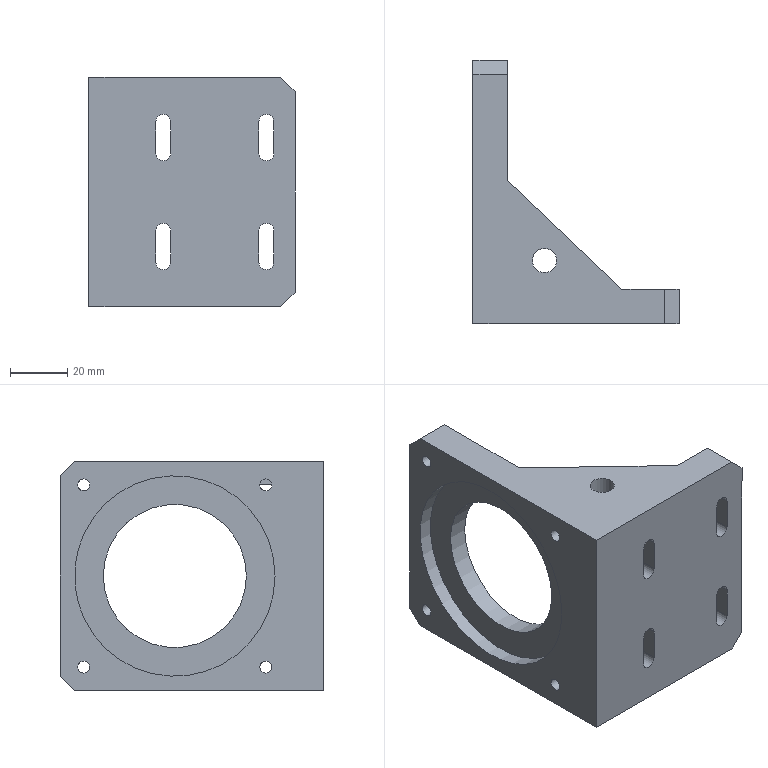Part | NX | 1 solid | 39 faces | box 72 x 92 x 80 mm | volume 113529 mm3 | plane 24 | cylinder 15 | commonest cylinder face diameters 5.2 x8 4.2 x4 8.5 x1 50 x1 70 x1
STEP:
#1=CARTESIAN_POINT('',(0.,65.,0.));
#2=VERTEX_POINT('',#1);
#3=CARTESIAN_POINT('',(0.,40.,0.));
#4=DIRECTION('',(1.,0.,0.));
#5=DIRECTION('',(0.,1.,0.));
#6=AXIS2_PLACEMENT_3D('',#3,#4,#5);
#7=CIRCLE('',#6,25.);
#8=EDGE_CURVE('',#2,#2,#7,.T.);
#9=ORIENTED_EDGE('',*,*,#8,.T.);
#10=EDGE_LOOP('',(#9));
#11=FACE_BOUND('',#10,.T.);
#12=CARTESIAN_POINT('',(-7.,15.,0.));
#13=VERTEX_POINT('',#12);
#14=CARTESIAN_POINT('',(-7.,40.,0.));
#15=DIRECTION('',(-1.,0.,0.));
#16=DIRECTION('',(0.,-1.,0.));
#17=AXIS2_PLACEMENT_3D('',#14,#15,#16);
#18=CIRCLE('',#17,25.);
#19=EDGE_CURVE('',#13,#13,#18,.F.);
#20=ORIENTED_EDGE('',*,*,#19,.F.);
#21=EDGE_LOOP('',(#20));
#22=FACE_BOUND('',#21,.T.);
#23=CARTESIAN_POINT('',(60.,40.,0.));
#24=DIRECTION('',(-1.,0.,0.));
#25=DIRECTION('',(0.,-1.,0.));
#26=AXIS2_PLACEMENT_3D('',#23,#24,#25);
#27=CYLINDRICAL_SURFACE('',#26,25.);
#28=ADVANCED_FACE('',(#11,#22),#27,.F.);
#29=CARTESIAN_POINT('',(0.,38.,32.));
#30=VERTEX_POINT('',#29);
#31=CARTESIAN_POINT('',(0.,10.272,32.));
#32=VERTEX_POINT('',#31);
#33=CARTESIAN_POINT('',(0.,80.,32.));
#34=DIRECTION('',(0.,-1.,0.));
#35=VECTOR('',#34,1000.);
#36=LINE('',#33,#35);
#37=EDGE_CURVE('',#30,#32,#36,.T.);
#38=ORIENTED_EDGE('',*,*,#37,.T.);
#39=CARTESIAN_POINT('',(0.,6.088,32.));
#40=VERTEX_POINT('',#39);
#41=CARTESIAN_POINT('',(0.,8.18,31.82));
#42=DIRECTION('',(1.,0.,0.));
#43=DIRECTION('',(0.,1.,0.));
#44=AXIS2_PLACEMENT_3D('',#41,#42,#43);
#45=CIRCLE('',#44,2.1);
#46=EDGE_CURVE('',#32,#40,#45,.F.);
#47=ORIENTED_EDGE('',*,*,#46,.T.);
#48=CARTESIAN_POINT('',(0.,0.,32.));
#49=VERTEX_POINT('',#48);
#50=CARTESIAN_POINT('',(0.,80.,32.));
#51=DIRECTION('',(0.,-1.,0.));
#52=VECTOR('',#51,1000.);
#53=LINE('',#50,#52);
#54=EDGE_CURVE('',#40,#49,#53,.T.);
#55=ORIENTED_EDGE('',*,*,#54,.T.);
#56=CARTESIAN_POINT('',(0.,0.,-40.));
#57=VERTEX_POINT('',#56);
#58=CARTESIAN_POINT('',(0.,0.,40.));
#59=DIRECTION('',(0.,0.,-1.));
#60=VECTOR('',#59,1000.);
#61=LINE('',#58,#60);
#62=EDGE_CURVE('',#49,#57,#61,.T.);
#63=ORIENTED_EDGE('',*,*,#62,.T.);
#64=CARTESIAN_POINT('',(0.,75.,-40.));
#65=VERTEX_POINT('',#64);
#66=CARTESIAN_POINT('',(0.,80.,-40.));
#67=DIRECTION('',(0.,-1.,0.));
#68=VECTOR('',#67,1000.);
#69=LINE('',#66,#68);
#70=EDGE_CURVE('',#65,#57,#69,.T.);
#71=ORIENTED_EDGE('',*,*,#70,.F.);
#72=CARTESIAN_POINT('',(0.,80.,-35.));
#73=VERTEX_POINT('',#72);
#74=CARTESIAN_POINT('',(0.,117.5,2.5));
#75=DIRECTION('',(0.,-0.7071,-0.7071));
#76=VECTOR('',#75,1000.);
#77=LINE('',#74,#76);
#78=EDGE_CURVE('',#65,#73,#77,.F.);
#79=ORIENTED_EDGE('',*,*,#78,.T.);
#80=CARTESIAN_POINT('',(0.,80.,35.));
#81=VERTEX_POINT('',#80);
#82=CARTESIAN_POINT('',(0.,80.,40.));
#83=DIRECTION('',(0.,0.,-1.));
#84=VECTOR('',#83,1000.);
#85=LINE('',#82,#84);
#86=EDGE_CURVE('',#81,#73,#85,.T.);
#87=ORIENTED_EDGE('',*,*,#86,.F.);
#88=CARTESIAN_POINT('',(0.,75.,40.));
#89=VERTEX_POINT('',#88);
#90=CARTESIAN_POINT('',(0.,77.5,37.5));
#91=DIRECTION('',(0.,-0.7071,0.7071));
#92=VECTOR('',#91,1000.);
#93=LINE('',#90,#92);
#94=EDGE_CURVE('',#81,#89,#93,.T.);
#95=ORIENTED_EDGE('',*,*,#94,.T.);
#96=CARTESIAN_POINT('',(0.,38.,40.));
#97=VERTEX_POINT('',#96);
#98=CARTESIAN_POINT('',(0.,80.,40.));
#99=DIRECTION('',(0.,-1.,0.));
#100=VECTOR('',#99,1000.);
#101=LINE('',#98,#100);
#102=EDGE_CURVE('',#89,#97,#101,.T.);
#103=ORIENTED_EDGE('',*,*,#102,.T.);
#104=CARTESIAN_POINT('',(0.,38.,40.));
#105=DIRECTION('',(0.,0.,-1.));
#106=VECTOR('',#105,1000.);
#107=LINE('',#104,#106);
#108=EDGE_CURVE('',#30,#97,#107,.F.);
#109=ORIENTED_EDGE('',*,*,#108,.F.);
#110=EDGE_LOOP('',(#38,#47,#55,#63,#71,#79,#87,#95,#103,#109));
#111=FACE_BOUND('',#110,.T.);
#112=CARTESIAN_POINT('',(0.,10.28,-31.82));
#113=VERTEX_POINT('',#112);
#114=CARTESIAN_POINT('',(0.,8.18,-31.82));
#115=DIRECTION('',(1.,0.,0.));
#116=DIRECTION('',(0.,1.,0.));
#117=AXIS2_PLACEMENT_3D('',#114,#115,#116);
#118=CIRCLE('',#117,2.1);
#119=EDGE_CURVE('',#113,#113,#118,.F.);
#120=ORIENTED_EDGE('',*,*,#119,.T.);
#121=EDGE_LOOP('',(#120));
#122=FACE_BOUND('',#121,.T.);
#123=ORIENTED_EDGE('',*,*,#8,.F.);
#124=EDGE_LOOP('',(#123));
#125=FACE_BOUND('',#124,.T.);
#126=CARTESIAN_POINT('',(0.,73.92,31.82));
#127=VERTEX_POINT('',#126);
#128=CARTESIAN_POINT('',(0.,71.82,31.82));
#129=DIRECTION('',(1.,0.,0.));
#130=DIRECTION('',(0.,1.,0.));
#131=AXIS2_PLACEMENT_3D('',#128,#129,#130);
#132=CIRCLE('',#131,2.1);
#133=EDGE_CURVE('',#127,#127,#132,.F.);
#134=ORIENTED_EDGE('',*,*,#133,.T.);
#135=EDGE_LOOP('',(#134));
#136=FACE_BOUND('',#135,.T.);
#137=CARTESIAN_POINT('',(0.,73.92,-31.82));
#138=VERTEX_POINT('',#137);
#139=CARTESIAN_POINT('',(0.,71.82,-31.82));
#140=DIRECTION('',(1.,0.,0.));
#141=DIRECTION('',(0.,1.,0.));
#142=AXIS2_PLACEMENT_3D('',#139,#140,#141);
#143=CIRCLE('',#142,2.1);
#144=EDGE_CURVE('',#138,#138,#143,.F.);
#145=ORIENTED_EDGE('',*,*,#144,.T.);
#146=EDGE_LOOP('',(#145));
#147=FACE_BOUND('',#146,.T.);
#148=CARTESIAN_POINT('',(0.,80.,40.));
#149=DIRECTION('',(1.,0.,0.));
#150=DIRECTION('',(0.,1.,0.));
#151=AXIS2_PLACEMENT_3D('',#148,#149,#150);
#152=PLANE('',#151);
#153=ADVANCED_FACE('',(#111,#122,#125,#136,#147),#152,.T.);
#154=CARTESIAN_POINT('',(52.6,-12.,24.5));
#155=VERTEX_POINT('',#154);
#156=CARTESIAN_POINT('',(52.6,-12.,13.5));
#157=VERTEX_POINT('',#156);
#158=CARTESIAN_POINT('',(52.6,-12.,13.5));
#159=DIRECTION('',(0.,0.,-1.));
#160=VECTOR('',#159,1000.);
#161=LINE('',#158,#160);
#162=EDGE_CURVE('',#155,#157,#161,.T.);
#163=ORIENTED_EDGE('',*,*,#162,.T.);
#164=CARTESIAN_POINT('',(47.4,-12.,13.5));
#165=VERTEX_POINT('',#164);
#166=CARTESIAN_POINT('',(50.,-12.,13.5));
#167=DIRECTION('',(0.,1.,0.));
#168=DIRECTION('',(0.,0.,1.));
#169=AXIS2_PLACEMENT_3D('',#166,#167,#168);
#170=CIRCLE('',#169,2.6);
#171=EDGE_CURVE('',#157,#165,#170,.T.);
#172=ORIENTED_EDGE('',*,*,#171,.T.);
#173=CARTESIAN_POINT('',(47.4,-12.,24.5));
#174=VERTEX_POINT('',#173);
#175=CARTESIAN_POINT('',(47.4,-12.,13.5));
#176=DIRECTION('',(0.,0.,1.));
#177=VECTOR('',#176,1000.);
#178=LINE('',#175,#177);
#179=EDGE_CURVE('',#165,#174,#178,.T.);
#180=ORIENTED_EDGE('',*,*,#179,.T.);
#181=CARTESIAN_POINT('',(50.,-12.,24.5));
#182=DIRECTION('',(0.,1.,0.));
#183=DIRECTION('',(0.,0.,1.));
#184=AXIS2_PLACEMENT_3D('',#181,#182,#183);
#185=CIRCLE('',#184,2.6);
#186=EDGE_CURVE('',#174,#155,#185,.T.);
#187=ORIENTED_EDGE('',*,*,#186,.T.);
#188=EDGE_LOOP('',(#163,#172,#180,#187));
#189=FACE_BOUND('',#188,.T.);
#190=CARTESIAN_POINT('',(16.6,-12.,24.5));
#191=VERTEX_POINT('',#190);
#192=CARTESIAN_POINT('',(16.6,-12.,13.5));
#193=VERTEX_POINT('',#192);
#194=CARTESIAN_POINT('',(16.6,-12.,13.5));
#195=DIRECTION('',(0.,0.,-1.));
#196=VECTOR('',#195,1000.);
#197=LINE('',#194,#196);
#198=EDGE_CURVE('',#191,#193,#197,.T.);
#199=ORIENTED_EDGE('',*,*,#198,.T.);
#200=CARTESIAN_POINT('',(11.4,-12.,13.5));
#201=VERTEX_POINT('',#200);
#202=CARTESIAN_POINT('',(14.,-12.,13.5));
#203=DIRECTION('',(0.,1.,0.));
#204=DIRECTION('',(0.,0.,1.));
#205=AXIS2_PLACEMENT_3D('',#202,#203,#204);
#206=CIRCLE('',#205,2.6);
#207=EDGE_CURVE('',#193,#201,#206,.T.);
#208=ORIENTED_EDGE('',*,*,#207,.T.);
#209=CARTESIAN_POINT('',(11.4,-12.,24.5));
#210=VERTEX_POINT('',#209);
#211=CARTESIAN_POINT('',(11.4,-12.,13.5));
#212=DIRECTION('',(0.,0.,1.));
#213=VECTOR('',#212,1000.);
#214=LINE('',#211,#213);
#215=EDGE_CURVE('',#201,#210,#214,.T.);
#216=ORIENTED_EDGE('',*,*,#215,.T.);
#217=CARTESIAN_POINT('',(14.,-12.,24.5));
#218=DIRECTION('',(0.,1.,0.));
#219=DIRECTION('',(0.,0.,1.));
#220=AXIS2_PLACEMENT_3D('',#217,#218,#219);
#221=CIRCLE('',#220,2.6);
#222=EDGE_CURVE('',#210,#191,#221,.T.);
#223=ORIENTED_EDGE('',*,*,#222,.T.);
#224=EDGE_LOOP('',(#199,#208,#216,#223));
#225=FACE_BOUND('',#224,.T.);
#226=CARTESIAN_POINT('',(47.4,-12.,-24.5));
#227=VERTEX_POINT('',#226);
#228=CARTESIAN_POINT('',(47.4,-12.,-13.5));
#229=VERTEX_POINT('',#228);
#230=CARTESIAN_POINT('',(47.4,-12.,-13.5));
#231=DIRECTION('',(0.,0.,1.));
#232=VECTOR('',#231,1000.);
#233=LINE('',#230,#232);
#234=EDGE_CURVE('',#227,#229,#233,.T.);
#235=ORIENTED_EDGE('',*,*,#234,.T.);
#236=CARTESIAN_POINT('',(52.6,-12.,-13.5));
#237=VERTEX_POINT('',#236);
#238=CARTESIAN_POINT('',(50.,-12.,-13.5));
#239=DIRECTION('',(0.,1.,0.));
#240=DIRECTION('',(0.,0.,1.));
#241=AXIS2_PLACEMENT_3D('',#238,#239,#240);
#242=CIRCLE('',#241,2.6);
#243=EDGE_CURVE('',#229,#237,#242,.T.);
#244=ORIENTED_EDGE('',*,*,#243,.T.);
#245=CARTESIAN_POINT('',(52.6,-12.,-24.5));
#246=VERTEX_POINT('',#245);
#247=CARTESIAN_POINT('',(52.6,-12.,-13.5));
#248=DIRECTION('',(0.,0.,-1.));
#249=VECTOR('',#248,1000.);
#250=LINE('',#247,#249);
#251=EDGE_CURVE('',#237,#246,#250,.T.);
#252=ORIENTED_EDGE('',*,*,#251,.T.);
#253=CARTESIAN_POINT('',(50.,-12.,-24.5));
#254=DIRECTION('',(0.,1.,0.));
#255=DIRECTION('',(0.,0.,1.));
#256=AXIS2_PLACEMENT_3D('',#253,#254,#255);
#257=CIRCLE('',#256,2.6);
#258=EDGE_CURVE('',#246,#227,#257,.T.);
#259=ORIENTED_EDGE('',*,*,#258,.T.);
#260=EDGE_LOOP('',(#235,#244,#252,#259));
#261=FACE_BOUND('',#260,.T.);
#262=CARTESIAN_POINT('',(16.6,-12.,-13.5));
#263=VERTEX_POINT('',#262);
#264=CARTESIAN_POINT('',(16.6,-12.,-24.5));
#265=VERTEX_POINT('',#264);
#266=CARTESIAN_POINT('',(16.6,-12.,-24.5));
#267=DIRECTION('',(0.,0.,-1.));
#268=VECTOR('',#267,1000.);
#269=LINE('',#266,#268);
#270=EDGE_CURVE('',#263,#265,#269,.T.);
#271=ORIENTED_EDGE('',*,*,#270,.T.);
#272=CARTESIAN_POINT('',(11.4,-12.,-24.5));
#273=VERTEX_POINT('',#272);
#274=CARTESIAN_POINT('',(14.,-12.,-24.5));
#275=DIRECTION('',(0.,1.,0.));
#276=DIRECTION('',(0.,0.,1.));
#277=AXIS2_PLACEMENT_3D('',#274,#275,#276);
#278=CIRCLE('',#277,2.6);
#279=EDGE_CURVE('',#265,#273,#278,.T.);
#280=ORIENTED_EDGE('',*,*,#279,.T.);
#281=CARTESIAN_POINT('',(11.4,-12.,-13.5));
#282=VERTEX_POINT('',#281);
#283=CARTESIAN_POINT('',(11.4,-12.,-24.5));
#284=DIRECTION('',(0.,0.,1.));
#285=VECTOR('',#284,1000.);
#286=LINE('',#283,#285);
#287=EDGE_CURVE('',#273,#282,#286,.T.);
#288=ORIENTED_EDGE('',*,*,#287,.T.);
#289=CARTESIAN_POINT('',(14.,-12.,-13.5));
#290=DIRECTION('',(0.,1.,0.));
#291=DIRECTION('',(0.,0.,1.));
#292=AXIS2_PLACEMENT_3D('',#289,#290,#291);
#293=CIRCLE('',#292,2.6);
#294=EDGE_CURVE('',#282,#263,#293,.T.);
#295=ORIENTED_EDGE('',*,*,#294,.T.);
#296=EDGE_LOOP('',(#271,#280,#288,#295));
#297=FACE_BOUND('',#296,.T.);
#298=CARTESIAN_POINT('',(60.,-12.,35.));
#299=VERTEX_POINT('',#298);
#300=CARTESIAN_POINT('',(55.,-12.,40.));
#301=VERTEX_POINT('',#300);
#302=CARTESIAN_POINT('',(60.,-12.,35.));
#303=DIRECTION('',(-0.7071,0.,0.7071));
#304=VECTOR('',#303,1000.);
#305=LINE('',#302,#304);
#306=EDGE_CURVE('',#299,#301,#305,.T.);
#307=ORIENTED_EDGE('',*,*,#306,.T.);
#308=CARTESIAN_POINT('',(-12.,-12.,40.));
#309=VERTEX_POINT('',#308);
#310=CARTESIAN_POINT('',(0.,-12.,40.));
#311=DIRECTION('',(1.,0.,0.));
#312=VECTOR('',#311,1000.);
#313=LINE('',#310,#312);
#314=EDGE_CURVE('',#309,#301,#313,.T.);
#315=ORIENTED_EDGE('',*,*,#314,.F.);
#316=CARTESIAN_POINT('',(-12.,-12.,-40.));
#317=VERTEX_POINT('',#316);
#318=CARTESIAN_POINT('',(-12.,-12.,40.));
#319=DIRECTION('',(0.,0.,-1.));
#320=VECTOR('',#319,1000.);
#321=LINE('',#318,#320);
#322=EDGE_CURVE('',#309,#317,#321,.T.);
#323=ORIENTED_EDGE('',*,*,#322,.T.);
#324=CARTESIAN_POINT('',(55.,-12.,-40.));
#325=VERTEX_POINT('',#324);
#326=CARTESIAN_POINT('',(0.,-12.,-40.));
#327=DIRECTION('',(1.,0.,0.));
#328=VECTOR('',#327,1000.);
#329=LINE('',#326,#328);
#330=EDGE_CURVE('',#317,#325,#329,.T.);
#331=ORIENTED_EDGE('',*,*,#330,.T.);
#332=CARTESIAN_POINT('',(60.,-12.,-35.));
#333=VERTEX_POINT('',#332);
#334=CARTESIAN_POINT('',(55.,-12.,-40.));
#335=DIRECTION('',(-0.7071,0.,-0.7071));
#336=VECTOR('',#335,1000.);
#337=LINE('',#334,#336);
#338=EDGE_CURVE('',#325,#333,#337,.F.);
#339=ORIENTED_EDGE('',*,*,#338,.T.);
#340=CARTESIAN_POINT('',(60.,-12.,40.));
#341=DIRECTION('',(0.,0.,-1.));
#342=VECTOR('',#341,1000.);
#343=LINE('',#340,#342);
#344=EDGE_CURVE('',#299,#333,#343,.T.);
#345=ORIENTED_EDGE('',*,*,#344,.F.);
#346=EDGE_LOOP('',(#307,#315,#323,#331,#339,#345));
#347=FACE_BOUND('',#346,.T.);
#348=CARTESIAN_POINT('',(0.,-12.,40.));
#349=DIRECTION('',(0.,1.,0.));
#350=DIRECTION('',(0.,0.,1.));
#351=AXIS2_PLACEMENT_3D('',#348,#349,#350);
#352=PLANE('',#351);
#353=ADVANCED_FACE('',(#189,#225,#261,#297,#347),#352,.F.);
#354=ORIENTED_EDGE('',*,*,#344,.T.);
#355=CARTESIAN_POINT('',(60.,0.,-35.));
#356=VERTEX_POINT('',#355);
#357=CARTESIAN_POINT('',(60.,0.,-35.));
#358=DIRECTION('',(0.,1.,0.));
#359=VECTOR('',#358,1000.);
#360=LINE('',#357,#359);
#361=EDGE_CURVE('',#333,#356,#360,.T.);
#362=ORIENTED_EDGE('',*,*,#361,.T.);
#363=CARTESIAN_POINT('',(60.,0.,35.));
#364=VERTEX_POINT('',#363);
#365=CARTESIAN_POINT('',(60.,0.,40.));
#366=DIRECTION('',(0.,0.,-1.));
#367=VECTOR('',#366,1000.);
#368=LINE('',#365,#367);
#369=EDGE_CURVE('',#364,#356,#368,.T.);
#370=ORIENTED_EDGE('',*,*,#369,.F.);
#371=CARTESIAN_POINT('',(60.,-12.,35.));
#372=DIRECTION('',(0.,-1.,0.));
#373=VECTOR('',#372,1000.);
#374=LINE('',#371,#373);
#375=EDGE_CURVE('',#364,#299,#374,.T.);
#376=ORIENTED_EDGE('',*,*,#375,.T.);
#377=EDGE_LOOP('',(#354,#362,#370,#376));
#378=FACE_BOUND('',#377,.T.);
#379=CARTESIAN_POINT('',(60.,0.,40.));
#380=DIRECTION('',(1.,0.,0.));
#381=DIRECTION('',(0.,0.,-1.));
#382=AXIS2_PLACEMENT_3D('',#379,#380,#381);
#383=PLANE('',#382);
#384=ADVANCED_FACE('',(#378),#383,.T.);
#385=CARTESIAN_POINT('',(40.,0.,40.));
#386=VERTEX_POINT('',#385);
#387=CARTESIAN_POINT('',(40.,0.,32.));
#388=VERTEX_POINT('',#387);
#389=CARTESIAN_POINT('',(40.,0.,40.));
#390=DIRECTION('',(0.,0.,1.));
#391=VECTOR('',#390,1000.);
#392=LINE('',#389,#391);
#393=EDGE_CURVE('',#386,#388,#392,.F.);
#394=ORIENTED_EDGE('',*,*,#393,.F.);
#395=CARTESIAN_POINT('',(55.,0.,40.));
#396=VERTEX_POINT('',#395);
#397=CARTESIAN_POINT('',(0.,0.,40.));
#398=DIRECTION('',(1.,0.,0.));
#399=VECTOR('',#398,1000.);
#400=LINE('',#397,#399);
#401=EDGE_CURVE('',#386,#396,#400,.T.);
#402=ORIENTED_EDGE('',*,*,#401,.T.);
#403=CARTESIAN_POINT('',(27.5,0.,67.5));
#404=DIRECTION('',(0.7071,0.,-0.7071));
#405=VECTOR('',#404,1000.);
#406=LINE('',#403,#405);
#407=EDGE_CURVE('',#396,#364,#406,.T.);
#408=ORIENTED_EDGE('',*,*,#407,.T.);
#409=ORIENTED_EDGE('',*,*,#369,.T.);
#410=CARTESIAN_POINT('',(55.,0.,-40.));
#411=VERTEX_POINT('',#410);
#412=CARTESIAN_POINT('',(67.5,0.,-27.5));
#413=DIRECTION('',(0.7071,0.,0.7071));
#414=VECTOR('',#413,1000.);
#415=LINE('',#412,#414);
#416=EDGE_CURVE('',#356,#411,#415,.F.);
#417=ORIENTED_EDGE('',*,*,#416,.T.);
#418=CARTESIAN_POINT('',(0.,0.,-40.));
#419=DIRECTION('',(1.,0.,0.));
#420=VECTOR('',#419,1000.);
#421=LINE('',#418,#420);
#422=EDGE_CURVE('',#57,#411,#421,.T.);
#423=ORIENTED_EDGE('',*,*,#422,.F.);
#424=ORIENTED_EDGE('',*,*,#62,.F.);
#425=CARTESIAN_POINT('',(0.,0.,32.));
#426=DIRECTION('',(1.,0.,0.));
#427=VECTOR('',#426,1000.);
#428=LINE('',#425,#427);
#429=EDGE_CURVE('',#49,#388,#428,.T.);
#430=ORIENTED_EDGE('',*,*,#429,.T.);
#431=EDGE_LOOP('',(#394,#402,#408,#409,#417,#423,#424,#430));
#432=FACE_BOUND('',#431,.T.);
#433=CARTESIAN_POINT('',(52.6,0.,13.5));
#434=VERTEX_POINT('',#433);
#435=CARTESIAN_POINT('',(47.4,0.,13.5));
#436=VERTEX_POINT('',#435);
#437=CARTESIAN_POINT('',(50.,0.,13.5));
#438=DIRECTION('',(0.,1.,0.));
#439=DIRECTION('',(0.,0.,1.));
#440=AXIS2_PLACEMENT_3D('',#437,#438,#439);
#441=CIRCLE('',#440,2.6);
#442=EDGE_CURVE('',#434,#436,#441,.T.);
#443=ORIENTED_EDGE('',*,*,#442,.F.);
#444=CARTESIAN_POINT('',(52.6,0.,24.5));
#445=VERTEX_POINT('',#444);
#446=CARTESIAN_POINT('',(52.6,0.,13.5));
#447=DIRECTION('',(0.,0.,-1.));
#448=VECTOR('',#447,1000.);
#449=LINE('',#446,#448);
#450=EDGE_CURVE('',#445,#434,#449,.T.);
#451=ORIENTED_EDGE('',*,*,#450,.F.);
#452=CARTESIAN_POINT('',(47.4,0.,24.5));
#453=VERTEX_POINT('',#452);
#454=CARTESIAN_POINT('',(50.,0.,24.5));
#455=DIRECTION('',(0.,1.,0.));
#456=DIRECTION('',(0.,0.,1.));
#457=AXIS2_PLACEMENT_3D('',#454,#455,#456);
#458=CIRCLE('',#457,2.6);
#459=EDGE_CURVE('',#453,#445,#458,.T.);
#460=ORIENTED_EDGE('',*,*,#459,.F.);
#461=CARTESIAN_POINT('',(47.4,0.,13.5));
#462=DIRECTION('',(0.,0.,1.));
#463=VECTOR('',#462,1000.);
#464=LINE('',#461,#463);
#465=EDGE_CURVE('',#436,#453,#464,.T.);
#466=ORIENTED_EDGE('',*,*,#465,.F.);
#467=EDGE_LOOP('',(#443,#451,#460,#466));
#468=FACE_BOUND('',#467,.T.);
#469=CARTESIAN_POINT('',(16.6,0.,13.5));
#470=VERTEX_POINT('',#469);
#471=CARTESIAN_POINT('',(11.4,0.,13.5));
#472=VERTEX_POINT('',#471);
#473=CARTESIAN_POINT('',(14.,0.,13.5));
#474=DIRECTION('',(0.,1.,0.));
#475=DIRECTION('',(0.,0.,1.));
#476=AXIS2_PLACEMENT_3D('',#473,#474,#475);
#477=CIRCLE('',#476,2.6);
#478=EDGE_CURVE('',#470,#472,#477,.T.);
#479=ORIENTED_EDGE('',*,*,#478,.F.);
#480=CARTESIAN_POINT('',(16.6,0.,24.5));
#481=VERTEX_POINT('',#480);
#482=CARTESIAN_POINT('',(16.6,0.,13.5));
#483=DIRECTION('',(0.,0.,-1.));
#484=VECTOR('',#483,1000.);
#485=LINE('',#482,#484);
#486=EDGE_CURVE('',#481,#470,#485,.T.);
#487=ORIENTED_EDGE('',*,*,#486,.F.);
#488=CARTESIAN_POINT('',(11.4,0.,24.5));
#489=VERTEX_POINT('',#488);
#490=CARTESIAN_POINT('',(14.,0.,24.5));
#491=DIRECTION('',(0.,1.,0.));
#492=DIRECTION('',(0.,0.,1.));
#493=AXIS2_PLACEMENT_3D('',#490,#491,#492);
#494=CIRCLE('',#493,2.6);
#495=EDGE_CURVE('',#489,#481,#494,.T.);
#496=ORIENTED_EDGE('',*,*,#495,.F.);
#497=CARTESIAN_POINT('',(11.4,0.,13.5));
#498=DIRECTION('',(0.,0.,1.));
#499=VECTOR('',#498,1000.);
#500=LINE('',#497,#499);
#501=EDGE_CURVE('',#472,#489,#500,.T.);
#502=ORIENTED_EDGE('',*,*,#501,.F.);
#503=EDGE_LOOP('',(#479,#487,#496,#502));
#504=FACE_BOUND('',#503,.T.);
#505=CARTESIAN_POINT('',(47.4,0.,-13.5));
#506=VERTEX_POINT('',#505);
#507=CARTESIAN_POINT('',(52.6,0.,-13.5));
#508=VERTEX_POINT('',#507);
#509=CARTESIAN_POINT('',(50.,0.,-13.5));
#510=DIRECTION('',(0.,1.,0.));
#511=DIRECTION('',(0.,0.,1.));
#512=AXIS2_PLACEMENT_3D('',#509,#510,#511);
#513=CIRCLE('',#512,2.6);
#514=EDGE_CURVE('',#506,#508,#513,.T.);
#515=ORIENTED_EDGE('',*,*,#514,.F.);
#516=CARTESIAN_POINT('',(47.4,0.,-24.5));
#517=VERTEX_POINT('',#516);
#518=CARTESIAN_POINT('',(47.4,0.,-13.5));
#519=DIRECTION('',(0.,0.,1.));
#520=VECTOR('',#519,1000.);
#521=LINE('',#518,#520);
#522=EDGE_CURVE('',#517,#506,#521,.T.);
#523=ORIENTED_EDGE('',*,*,#522,.F.);
#524=CARTESIAN_POINT('',(52.6,0.,-24.5));
#525=VERTEX_POINT('',#524);
#526=CARTESIAN_POINT('',(50.,0.,-24.5));
#527=DIRECTION('',(0.,1.,0.));
#528=DIRECTION('',(0.,0.,1.));
#529=AXIS2_PLACEMENT_3D('',#526,#527,#528);
#530=CIRCLE('',#529,2.6);
#531=EDGE_CURVE('',#525,#517,#530,.T.);
#532=ORIENTED_EDGE('',*,*,#531,.F.);
#533=CARTESIAN_POINT('',(52.6,0.,-13.5));
#534=DIRECTION('',(0.,0.,-1.));
#535=VECTOR('',#534,1000.);
#536=LINE('',#533,#535);
#537=EDGE_CURVE('',#508,#525,#536,.T.);
#538=ORIENTED_EDGE('',*,*,#537,.F.);
#539=EDGE_LOOP('',(#515,#523,#532,#538));
#540=FACE_BOUND('',#539,.T.);
#541=CARTESIAN_POINT('',(16.6,0.,-24.5));
#542=VERTEX_POINT('',#541);
#543=CARTESIAN_POINT('',(11.4,0.,-24.5));
#544=VERTEX_POINT('',#543);
#545=CARTESIAN_POINT('',(14.,0.,-24.5));
#546=DIRECTION('',(0.,1.,0.));
#547=DIRECTION('',(0.,0.,1.));
#548=AXIS2_PLACEMENT_3D('',#545,#546,#547);
#549=CIRCLE('',#548,2.6);
#550=EDGE_CURVE('',#542,#544,#549,.T.);
#551=ORIENTED_EDGE('',*,*,#550,.F.);
#552=CARTESIAN_POINT('',(16.6,0.,-13.5));
#553=VERTEX_POINT('',#552);
#554=CARTESIAN_POINT('',(16.6,0.,-24.5));
#555=DIRECTION('',(0.,0.,-1.));
#556=VECTOR('',#555,1000.);
#557=LINE('',#554,#556);
#558=EDGE_CURVE('',#553,#542,#557,.T.);
#559=ORIENTED_EDGE('',*,*,#558,.F.);
#560=CARTESIAN_POINT('',(11.4,0.,-13.5));
#561=VERTEX_POINT('',#560);
#562=CARTESIAN_POINT('',(14.,0.,-13.5));
#563=DIRECTION('',(0.,1.,0.));
#564=DIRECTION('',(0.,0.,1.));
#565=AXIS2_PLACEMENT_3D('',#562,#563,#564);
#566=CIRCLE('',#565,2.6);
#567=EDGE_CURVE('',#561,#553,#566,.T.);
#568=ORIENTED_EDGE('',*,*,#567,.F.);
#569=CARTESIAN_POINT('',(11.4,0.,-24.5));
#570=DIRECTION('',(0.,0.,1.));
#571=VECTOR('',#570,1000.);
#572=LINE('',#569,#571);
#573=EDGE_CURVE('',#544,#561,#572,.T.);
#574=ORIENTED_EDGE('',*,*,#573,.F.);
#575=EDGE_LOOP('',(#551,#559,#568,#574));
#576=FACE_BOUND('',#575,.T.);
#577=CARTESIAN_POINT('',(0.,0.,40.));
#578=DIRECTION('',(0.,1.,0.));
#579=DIRECTION('',(0.,0.,1.));
#580=AXIS2_PLACEMENT_3D('',#577,#578,#579);
#581=PLANE('',#580);
#582=ADVANCED_FACE('',(#432,#468,#504,#540,#576),#581,.T.);
#583=ORIENTED_EDGE('',*,*,#86,.T.);
#584=CARTESIAN_POINT('',(-12.,80.,-35.));
#585=VERTEX_POINT('',#584);
#586=CARTESIAN_POINT('',(-12.,80.,-35.));
#587=DIRECTION('',(-1.,0.,0.));
#588=VECTOR('',#587,1000.);
#589=LINE('',#586,#588);
#590=EDGE_CURVE('',#73,#585,#589,.T.);
#591=ORIENTED_EDGE('',*,*,#590,.T.);
#592=CARTESIAN_POINT('',(-12.,80.,35.));
#593=VERTEX_POINT('',#592);
#594=CARTESIAN_POINT('',(-12.,80.,40.));
#595=DIRECTION('',(0.,0.,-1.));
#596=VECTOR('',#595,1000.);
#597=LINE('',#594,#596);
#598=EDGE_CURVE('',#593,#585,#597,.T.);
#599=ORIENTED_EDGE('',*,*,#598,.F.);
#600=CARTESIAN_POINT('',(0.,80.,35.));
#601=DIRECTION('',(1.,0.,0.));
#602=VECTOR('',#601,1000.);
#603=LINE('',#600,#602);
#604=EDGE_CURVE('',#593,#81,#603,.T.);
#605=ORIENTED_EDGE('',*,*,#604,.T.);
#606=EDGE_LOOP('',(#583,#591,#599,#605));
#607=FACE_BOUND('',#606,.T.);
#608=CARTESIAN_POINT('',(-12.,80.,40.));
#609=DIRECTION('',(0.,1.,0.));
#610=DIRECTION('',(0.,0.,1.));
#611=AXIS2_PLACEMENT_3D('',#608,#609,#610);
#612=PLANE('',#611);
#613=ADVANCED_FACE('',(#607),#612,.T.);
#614=CARTESIAN_POINT('',(-12.,5.,0.));
#615=VERTEX_POINT('',#614);
#616=CARTESIAN_POINT('',(-12.,40.,0.));
#617=DIRECTION('',(-1.,0.,0.));
#618=DIRECTION('',(0.,-1.,0.));
#619=AXIS2_PLACEMENT_3D('',#616,#617,#618);
#620=CIRCLE('',#619,35.);
#621=EDGE_CURVE('',#615,#615,#620,.T.);
#622=ORIENTED_EDGE('',*,*,#621,.F.);
#623=EDGE_LOOP('',(#622));
#624=FACE_BOUND('',#623,.T.);
#625=CARTESIAN_POINT('',(-12.,71.82,-29.72));
#626=VERTEX_POINT('',#625);
#627=CARTESIAN_POINT('',(-12.,71.82,-31.82));
#628=DIRECTION('',(-1.,0.,0.));
#629=DIRECTION('',(0.,0.,1.));
#630=AXIS2_PLACEMENT_3D('',#627,#628,#629);
#631=CIRCLE('',#630,2.1);
#632=EDGE_CURVE('',#626,#626,#631,.T.);
#633=ORIENTED_EDGE('',*,*,#632,.F.);
#634=EDGE_LOOP('',(#633));
#635=FACE_BOUND('',#634,.T.);
#636=CARTESIAN_POINT('',(-12.,71.82,33.92));
#637=VERTEX_POINT('',#636);
#638=CARTESIAN_POINT('',(-12.,71.82,31.82));
#639=DIRECTION('',(-1.,0.,0.));
#640=DIRECTION('',(0.,0.,1.));
#641=AXIS2_PLACEMENT_3D('',#638,#639,#640);
#642=CIRCLE('',#641,2.1);
#643=EDGE_CURVE('',#637,#637,#642,.T.);
#644=ORIENTED_EDGE('',*,*,#643,.F.);
#645=EDGE_LOOP('',(#644));
#646=FACE_BOUND('',#645,.T.);
#647=CARTESIAN_POINT('',(-12.,8.18,33.92));
#648=VERTEX_POINT('',#647);
#649=CARTESIAN_POINT('',(-12.,8.18,31.82));
#650=DIRECTION('',(-1.,0.,0.));
#651=DIRECTION('',(0.,0.,1.));
#652=AXIS2_PLACEMENT_3D('',#649,#650,#651);
#653=CIRCLE('',#652,2.1);
#654=EDGE_CURVE('',#648,#648,#653,.T.);
#655=ORIENTED_EDGE('',*,*,#654,.F.);
#656=EDGE_LOOP('',(#655));
#657=FACE_BOUND('',#656,.T.);
#658=CARTESIAN_POINT('',(-12.,8.18,-29.72));
#659=VERTEX_POINT('',#658);
#660=CARTESIAN_POINT('',(-12.,8.18,-31.82));
#661=DIRECTION('',(-1.,0.,0.));
#662=DIRECTION('',(0.,0.,1.));
#663=AXIS2_PLACEMENT_3D('',#660,#661,#662);
#664=CIRCLE('',#663,2.1);
#665=EDGE_CURVE('',#659,#659,#664,.T.);
#666=ORIENTED_EDGE('',*,*,#665,.F.);
#667=EDGE_LOOP('',(#666));
#668=FACE_BOUND('',#667,.T.);
#669=ORIENTED_EDGE('',*,*,#322,.F.);
#670=CARTESIAN_POINT('',(-12.,75.,40.));
#671=VERTEX_POINT('',#670);
#672=CARTESIAN_POINT('',(-12.,80.,40.));
#673=DIRECTION('',(0.,-1.,0.));
#674=VECTOR('',#673,1000.);
#675=LINE('',#672,#674);
#676=EDGE_CURVE('',#671,#309,#675,.T.);
#677=ORIENTED_EDGE('',*,*,#676,.F.);
#678=CARTESIAN_POINT('',(-12.,80.,35.));
#679=DIRECTION('',(0.,0.7071,-0.7071));
#680=VECTOR('',#679,1000.);
#681=LINE('',#678,#680);
#682=EDGE_CURVE('',#671,#593,#681,.T.);
#683=ORIENTED_EDGE('',*,*,#682,.T.);
#684=ORIENTED_EDGE('',*,*,#598,.T.);
#685=CARTESIAN_POINT('',(-12.,75.,-40.));
#686=VERTEX_POINT('',#685);
#687=CARTESIAN_POINT('',(-12.,75.,-40.));
#688=DIRECTION('',(0.,0.7071,0.7071));
#689=VECTOR('',#688,1000.);
#690=LINE('',#687,#689);
#691=EDGE_CURVE('',#585,#686,#690,.F.);
#692=ORIENTED_EDGE('',*,*,#691,.T.);
#693=CARTESIAN_POINT('',(-12.,80.,-40.));
#694=DIRECTION('',(0.,-1.,0.));
#695=VECTOR('',#694,1000.);
#696=LINE('',#693,#695);
#697=EDGE_CURVE('',#686,#317,#696,.T.);
#698=ORIENTED_EDGE('',*,*,#697,.T.);
#699=EDGE_LOOP('',(#669,#677,#683,#684,#692,#698));
#700=FACE_BOUND('',#699,.T.);
#701=CARTESIAN_POINT('',(-12.,80.,40.));
#702=DIRECTION('',(1.,0.,0.));
#703=DIRECTION('',(0.,1.,0.));
#704=AXIS2_PLACEMENT_3D('',#701,#702,#703);
#705=PLANE('',#704);
#706=ADVANCED_FACE('',(#624,#635,#646,#657,#668,#700),#705,.F.);
#707=CARTESIAN_POINT('',(17.25,10.,40.));
#708=VERTEX_POINT('',#707);
#709=CARTESIAN_POINT('',(13.,10.,40.));
#710=DIRECTION('',(0.,0.,1.));
#711=DIRECTION('',(1.,0.,0.));
#712=AXIS2_PLACEMENT_3D('',#709,#710,#711);
#713=CIRCLE('',#712,4.25);
#714=EDGE_CURVE('',#708,#708,#713,.T.);
#715=ORIENTED_EDGE('',*,*,#714,.F.);
#716=EDGE_LOOP('',(#715));
#717=FACE_BOUND('',#716,.T.);
#718=ORIENTED_EDGE('',*,*,#401,.F.);
#719=CARTESIAN_POINT('',(0.,38.,40.));
#720=DIRECTION('',(0.725,-0.6887,0.));
#721=VECTOR('',#720,1000.);
#722=LINE('',#719,#721);
#723=EDGE_CURVE('',#97,#386,#722,.T.);
#724=ORIENTED_EDGE('',*,*,#723,.F.);
#725=ORIENTED_EDGE('',*,*,#102,.F.);
#726=CARTESIAN_POINT('',(-12.,75.,40.));
#727=DIRECTION('',(-1.,0.,0.));
#728=VECTOR('',#727,1000.);
#729=LINE('',#726,#728);
#730=EDGE_CURVE('',#89,#671,#729,.T.);
#731=ORIENTED_EDGE('',*,*,#730,.T.);
#732=ORIENTED_EDGE('',*,*,#676,.T.);
#733=ORIENTED_EDGE('',*,*,#314,.T.);
#734=CARTESIAN_POINT('',(55.,0.,40.));
#735=DIRECTION('',(0.,1.,0.));
#736=VECTOR('',#735,1000.);
#737=LINE('',#734,#736);
#738=EDGE_CURVE('',#301,#396,#737,.T.);
#739=ORIENTED_EDGE('',*,*,#738,.T.);
#740=EDGE_LOOP('',(#718,#724,#725,#731,#732,#733,#739));
#741=FACE_BOUND('',#740,.T.);
#742=CARTESIAN_POINT('',(0.,0.,40.));
#743=DIRECTION('',(0.,0.,-1.));
#744=DIRECTION('',(-1.,0.,0.));
#745=AXIS2_PLACEMENT_3D('',#742,#743,#744);
#746=PLANE('',#745);
#747=ADVANCED_FACE('',(#717,#741),#746,.F.);
#748=ORIENTED_EDGE('',*,*,#697,.F.);
#749=CARTESIAN_POINT('',(0.,75.,-40.));
#750=DIRECTION('',(1.,0.,0.));
#751=VECTOR('',#750,1000.);
#752=LINE('',#749,#751);
#753=EDGE_CURVE('',#686,#65,#752,.T.);
#754=ORIENTED_EDGE('',*,*,#753,.T.);
#755=ORIENTED_EDGE('',*,*,#70,.T.);
#756=ORIENTED_EDGE('',*,*,#422,.T.);
#757=CARTESIAN_POINT('',(55.,0.,-40.));
#758=DIRECTION('',(0.,-1.,0.));
#759=VECTOR('',#758,1000.);
#760=LINE('',#757,#759);
#761=EDGE_CURVE('',#411,#325,#760,.T.);
#762=ORIENTED_EDGE('',*,*,#761,.T.);
#763=ORIENTED_EDGE('',*,*,#330,.F.);
#764=EDGE_LOOP('',(#748,#754,#755,#756,#762,#763));
#765=FACE_BOUND('',#764,.T.);
#766=CARTESIAN_POINT('',(0.,0.,-40.));
#767=DIRECTION('',(0.,0.,-1.));
#768=DIRECTION('',(-1.,0.,0.));
#769=AXIS2_PLACEMENT_3D('',#766,#767,#768);
#770=PLANE('',#769);
#771=ADVANCED_FACE('',(#765),#770,.T.);
#772=ORIENTED_EDGE('',*,*,#550,.T.);
#773=CARTESIAN_POINT('',(11.4,-12.,-24.5));
#774=DIRECTION('',(0.,1.,0.));
#775=VECTOR('',#774,1000.);
#776=LINE('',#773,#775);
#777=EDGE_CURVE('',#273,#544,#776,.T.);
#778=ORIENTED_EDGE('',*,*,#777,.F.);
#779=ORIENTED_EDGE('',*,*,#279,.F.);
#780=CARTESIAN_POINT('',(16.6,-12.,-24.5));
#781=DIRECTION('',(0.,1.,0.));
#782=VECTOR('',#781,1000.);
#783=LINE('',#780,#782);
#784=EDGE_CURVE('',#265,#542,#783,.T.);
#785=ORIENTED_EDGE('',*,*,#784,.T.);
#786=EDGE_LOOP('',(#772,#778,#779,#785));
#787=FACE_BOUND('',#786,.T.);
#788=CARTESIAN_POINT('',(14.,-12.,-24.5));
#789=DIRECTION('',(0.,1.,0.));
#790=DIRECTION('',(0.,0.,1.));
#791=AXIS2_PLACEMENT_3D('',#788,#789,#790);
#792=CYLINDRICAL_SURFACE('',#791,2.6);
#793=ADVANCED_FACE('',(#787),#792,.F.);
#794=ORIENTED_EDGE('',*,*,#558,.T.);
#795=ORIENTED_EDGE('',*,*,#784,.F.);
#796=ORIENTED_EDGE('',*,*,#270,.F.);
#797=CARTESIAN_POINT('',(16.6,-12.,-13.5));
#798=DIRECTION('',(0.,1.,0.));
#799=VECTOR('',#798,1000.);
#800=LINE('',#797,#799);
#801=EDGE_CURVE('',#263,#553,#800,.T.);
#802=ORIENTED_EDGE('',*,*,#801,.T.);
#803=EDGE_LOOP('',(#794,#795,#796,#802));
#804=FACE_BOUND('',#803,.T.);
#805=CARTESIAN_POINT('',(16.6,-12.,-24.5));
#806=DIRECTION('',(1.,0.,0.));
#807=DIRECTION('',(0.,0.,-1.));
#808=AXIS2_PLACEMENT_3D('',#805,#806,#807);
#809=PLANE('',#808);
#810=ADVANCED_FACE('',(#804),#809,.F.);
#811=ORIENTED_EDGE('',*,*,#567,.T.);
#812=ORIENTED_EDGE('',*,*,#801,.F.);
#813=ORIENTED_EDGE('',*,*,#294,.F.);
#814=CARTESIAN_POINT('',(11.4,-12.,-13.5));
#815=DIRECTION('',(0.,1.,0.));
#816=VECTOR('',#815,1000.);
#817=LINE('',#814,#816);
#818=EDGE_CURVE('',#282,#561,#817,.T.);
#819=ORIENTED_EDGE('',*,*,#818,.T.);
#820=EDGE_LOOP('',(#811,#812,#813,#819));
#821=FACE_BOUND('',#820,.T.);
#822=CARTESIAN_POINT('',(14.,-12.,-13.5));
#823=DIRECTION('',(0.,1.,0.));
#824=DIRECTION('',(0.,0.,1.));
#825=AXIS2_PLACEMENT_3D('',#822,#823,#824);
#826=CYLINDRICAL_SURFACE('',#825,2.6);
#827=ADVANCED_FACE('',(#821),#826,.F.);
#828=ORIENTED_EDGE('',*,*,#573,.T.);
#829=ORIENTED_EDGE('',*,*,#818,.F.);
#830=ORIENTED_EDGE('',*,*,#287,.F.);
#831=ORIENTED_EDGE('',*,*,#777,.T.);
#832=EDGE_LOOP('',(#828,#829,#830,#831));
#833=FACE_BOUND('',#832,.T.);
#834=CARTESIAN_POINT('',(11.4,-12.,-24.5));
#835=DIRECTION('',(-1.,0.,0.));
#836=DIRECTION('',(0.,0.,1.));
#837=AXIS2_PLACEMENT_3D('',#834,#835,#836);
#838=PLANE('',#837);
#839=ADVANCED_FACE('',(#833),#838,.F.);
#840=ORIENTED_EDGE('',*,*,#514,.T.);
#841=CARTESIAN_POINT('',(52.6,-12.,-13.5));
#842=DIRECTION('',(0.,1.,0.));
#843=VECTOR('',#842,1000.);
#844=LINE('',#841,#843);
#845=EDGE_CURVE('',#237,#508,#844,.T.);
#846=ORIENTED_EDGE('',*,*,#845,.F.);
#847=ORIENTED_EDGE('',*,*,#243,.F.);
#848=CARTESIAN_POINT('',(47.4,-12.,-13.5));
#849=DIRECTION('',(0.,1.,0.));
#850=VECTOR('',#849,1000.);
#851=LINE('',#848,#850);
#852=EDGE_CURVE('',#229,#506,#851,.T.);
#853=ORIENTED_EDGE('',*,*,#852,.T.);
#854=EDGE_LOOP('',(#840,#846,#847,#853));
#855=FACE_BOUND('',#854,.T.);
#856=CARTESIAN_POINT('',(50.,-12.,-13.5));
#857=DIRECTION('',(0.,1.,0.));
#858=DIRECTION('',(0.,0.,1.));
#859=AXIS2_PLACEMENT_3D('',#856,#857,#858);
#860=CYLINDRICAL_SURFACE('',#859,2.6);
#861=ADVANCED_FACE('',(#855),#860,.F.);
#862=ORIENTED_EDGE('',*,*,#522,.T.);
#863=ORIENTED_EDGE('',*,*,#852,.F.);
#864=ORIENTED_EDGE('',*,*,#234,.F.);
#865=CARTESIAN_POINT('',(47.4,-12.,-24.5));
#866=DIRECTION('',(0.,1.,0.));
#867=VECTOR('',#866,1000.);
#868=LINE('',#865,#867);
#869=EDGE_CURVE('',#227,#517,#868,.T.);
#870=ORIENTED_EDGE('',*,*,#869,.T.);
#871=EDGE_LOOP('',(#862,#863,#864,#870));
#872=FACE_BOUND('',#871,.T.);
#873=CARTESIAN_POINT('',(47.4,-12.,-13.5));
#874=DIRECTION('',(-1.,0.,0.));
#875=DIRECTION('',(0.,0.,1.));
#876=AXIS2_PLACEMENT_3D('',#873,#874,#875);
#877=PLANE('',#876);
#878=ADVANCED_FACE('',(#872),#877,.F.);
#879=ORIENTED_EDGE('',*,*,#531,.T.);
#880=ORIENTED_EDGE('',*,*,#869,.F.);
#881=ORIENTED_EDGE('',*,*,#258,.F.);
#882=CARTESIAN_POINT('',(52.6,-12.,-24.5));
#883=DIRECTION('',(0.,1.,0.));
#884=VECTOR('',#883,1000.);
#885=LINE('',#882,#884);
#886=EDGE_CURVE('',#246,#525,#885,.T.);
#887=ORIENTED_EDGE('',*,*,#886,.T.);
#888=EDGE_LOOP('',(#879,#880,#881,#887));
#889=FACE_BOUND('',#888,.T.);
#890=CARTESIAN_POINT('',(50.,-12.,-24.5));
#891=DIRECTION('',(0.,1.,0.));
#892=DIRECTION('',(0.,0.,1.));
#893=AXIS2_PLACEMENT_3D('',#890,#891,#892);
#894=CYLINDRICAL_SURFACE('',#893,2.6);
#895=ADVANCED_FACE('',(#889),#894,.F.);
#896=ORIENTED_EDGE('',*,*,#537,.T.);
#897=ORIENTED_EDGE('',*,*,#886,.F.);
#898=ORIENTED_EDGE('',*,*,#251,.F.);
#899=ORIENTED_EDGE('',*,*,#845,.T.);
#900=EDGE_LOOP('',(#896,#897,#898,#899));
#901=FACE_BOUND('',#900,.T.);
#902=CARTESIAN_POINT('',(52.6,-12.,-13.5));
#903=DIRECTION('',(1.,0.,0.));
#904=DIRECTION('',(0.,0.,-1.));
#905=AXIS2_PLACEMENT_3D('',#902,#903,#904);
#906=PLANE('',#905);
#907=ADVANCED_FACE('',(#901),#906,.F.);
#908=ORIENTED_EDGE('',*,*,#478,.T.);
#909=CARTESIAN_POINT('',(11.4,-12.,13.5));
#910=DIRECTION('',(0.,1.,0.));
#911=VECTOR('',#910,1000.);
#912=LINE('',#909,#911);
#913=EDGE_CURVE('',#201,#472,#912,.T.);
#914=ORIENTED_EDGE('',*,*,#913,.F.);
#915=ORIENTED_EDGE('',*,*,#207,.F.);
#916=CARTESIAN_POINT('',(16.6,-12.,13.5));
#917=DIRECTION('',(0.,1.,0.));
#918=VECTOR('',#917,1000.);
#919=LINE('',#916,#918);
#920=EDGE_CURVE('',#193,#470,#919,.T.);
#921=ORIENTED_EDGE('',*,*,#920,.T.);
#922=EDGE_LOOP('',(#908,#914,#915,#921));
#923=FACE_BOUND('',#922,.T.);
#924=CARTESIAN_POINT('',(14.,-12.,13.5));
#925=DIRECTION('',(0.,1.,0.));
#926=DIRECTION('',(0.,0.,1.));
#927=AXIS2_PLACEMENT_3D('',#924,#925,#926);
#928=CYLINDRICAL_SURFACE('',#927,2.6);
#929=ADVANCED_FACE('',(#923),#928,.F.);
#930=ORIENTED_EDGE('',*,*,#486,.T.);
#931=ORIENTED_EDGE('',*,*,#920,.F.);
#932=ORIENTED_EDGE('',*,*,#198,.F.);
#933=CARTESIAN_POINT('',(16.6,-12.,24.5));
#934=DIRECTION('',(0.,1.,0.));
#935=VECTOR('',#934,1000.);
#936=LINE('',#933,#935);
#937=EDGE_CURVE('',#191,#481,#936,.T.);
#938=ORIENTED_EDGE('',*,*,#937,.T.);
#939=EDGE_LOOP('',(#930,#931,#932,#938));
#940=FACE_BOUND('',#939,.T.);
#941=CARTESIAN_POINT('',(16.6,-12.,13.5));
#942=DIRECTION('',(1.,0.,0.));
#943=DIRECTION('',(0.,0.,-1.));
#944=AXIS2_PLACEMENT_3D('',#941,#942,#943);
#945=PLANE('',#944);
#946=ADVANCED_FACE('',(#940),#945,.F.);
#947=ORIENTED_EDGE('',*,*,#495,.T.);
#948=ORIENTED_EDGE('',*,*,#937,.F.);
#949=ORIENTED_EDGE('',*,*,#222,.F.);
#950=CARTESIAN_POINT('',(11.4,-12.,24.5));
#951=DIRECTION('',(0.,1.,0.));
#952=VECTOR('',#951,1000.);
#953=LINE('',#950,#952);
#954=EDGE_CURVE('',#210,#489,#953,.T.);
#955=ORIENTED_EDGE('',*,*,#954,.T.);
#956=EDGE_LOOP('',(#947,#948,#949,#955));
#957=FACE_BOUND('',#956,.T.);
#958=CARTESIAN_POINT('',(14.,-12.,24.5));
#959=DIRECTION('',(0.,1.,0.));
#960=DIRECTION('',(0.,0.,1.));
#961=AXIS2_PLACEMENT_3D('',#958,#959,#960);
#962=CYLINDRICAL_SURFACE('',#961,2.6);
#963=ADVANCED_FACE('',(#957),#962,.F.);
#964=ORIENTED_EDGE('',*,*,#501,.T.);
#965=ORIENTED_EDGE('',*,*,#954,.F.);
#966=ORIENTED_EDGE('',*,*,#215,.F.);
#967=ORIENTED_EDGE('',*,*,#913,.T.);
#968=EDGE_LOOP('',(#964,#965,#966,#967));
#969=FACE_BOUND('',#968,.T.);
#970=CARTESIAN_POINT('',(11.4,-12.,13.5));
#971=DIRECTION('',(-1.,0.,0.));
#972=DIRECTION('',(0.,0.,1.));
#973=AXIS2_PLACEMENT_3D('',#970,#971,#972);
#974=PLANE('',#973);
#975=ADVANCED_FACE('',(#969),#974,.F.);
#976=ORIENTED_EDGE('',*,*,#442,.T.);
#977=CARTESIAN_POINT('',(47.4,-12.,13.5));
#978=DIRECTION('',(0.,1.,0.));
#979=VECTOR('',#978,1000.);
#980=LINE('',#977,#979);
#981=EDGE_CURVE('',#165,#436,#980,.T.);
#982=ORIENTED_EDGE('',*,*,#981,.F.);
#983=ORIENTED_EDGE('',*,*,#171,.F.);
#984=CARTESIAN_POINT('',(52.6,-12.,13.5));
#985=DIRECTION('',(0.,1.,0.));
#986=VECTOR('',#985,1000.);
#987=LINE('',#984,#986);
#988=EDGE_CURVE('',#157,#434,#987,.T.);
#989=ORIENTED_EDGE('',*,*,#988,.T.);
#990=EDGE_LOOP('',(#976,#982,#983,#989));
#991=FACE_BOUND('',#990,.T.);
#992=CARTESIAN_POINT('',(50.,-12.,13.5));
#993=DIRECTION('',(0.,1.,0.));
#994=DIRECTION('',(0.,0.,1.));
#995=AXIS2_PLACEMENT_3D('',#992,#993,#994);
#996=CYLINDRICAL_SURFACE('',#995,2.6);
#997=ADVANCED_FACE('',(#991),#996,.F.);
#998=ORIENTED_EDGE('',*,*,#450,.T.);
#999=ORIENTED_EDGE('',*,*,#988,.F.);
#1000=ORIENTED_EDGE('',*,*,#162,.F.);
#1001=CARTESIAN_POINT('',(52.6,-12.,24.5));
#1002=DIRECTION('',(0.,1.,0.));
#1003=VECTOR('',#1002,1000.);
#1004=LINE('',#1001,#1003);
#1005=EDGE_CURVE('',#155,#445,#1004,.T.);
#1006=ORIENTED_EDGE('',*,*,#1005,.T.);
#1007=EDGE_LOOP('',(#998,#999,#1000,#1006));
#1008=FACE_BOUND('',#1007,.T.);
#1009=CARTESIAN_POINT('',(52.6,-12.,13.5));
#1010=DIRECTION('',(1.,0.,0.));
#1011=DIRECTION('',(0.,0.,-1.));
#1012=AXIS2_PLACEMENT_3D('',#1009,#1010,#1011);
#1013=PLANE('',#1012);
#1014=ADVANCED_FACE('',(#1008),#1013,.F.);
#1015=ORIENTED_EDGE('',*,*,#459,.T.);
#1016=ORIENTED_EDGE('',*,*,#1005,.F.);
#1017=ORIENTED_EDGE('',*,*,#186,.F.);
#1018=CARTESIAN_POINT('',(47.4,-12.,24.5));
#1019=DIRECTION('',(0.,1.,0.));
#1020=VECTOR('',#1019,1000.);
#1021=LINE('',#1018,#1020);
#1022=EDGE_CURVE('',#174,#453,#1021,.T.);
#1023=ORIENTED_EDGE('',*,*,#1022,.T.);
#1024=EDGE_LOOP('',(#1015,#1016,#1017,#1023));
#1025=FACE_BOUND('',#1024,.T.);
#1026=CARTESIAN_POINT('',(50.,-12.,24.5));
#1027=DIRECTION('',(0.,1.,0.));
#1028=DIRECTION('',(0.,0.,1.));
#1029=AXIS2_PLACEMENT_3D('',#1026,#1027,#1028);
#1030=CYLINDRICAL_SURFACE('',#1029,2.6);
#1031=ADVANCED_FACE('',(#1025),#1030,.F.);
#1032=ORIENTED_EDGE('',*,*,#465,.T.);
#1033=ORIENTED_EDGE('',*,*,#1022,.F.);
#1034=ORIENTED_EDGE('',*,*,#179,.F.);
#1035=ORIENTED_EDGE('',*,*,#981,.T.);
#1036=EDGE_LOOP('',(#1032,#1033,#1034,#1035));
#1037=FACE_BOUND('',#1036,.T.);
#1038=CARTESIAN_POINT('',(47.4,-12.,13.5));
#1039=DIRECTION('',(-1.,0.,0.));
#1040=DIRECTION('',(0.,0.,1.));
#1041=AXIS2_PLACEMENT_3D('',#1038,#1039,#1040);
#1042=PLANE('',#1041);
#1043=ADVANCED_FACE('',(#1037),#1042,.F.);
#1044=ORIENTED_EDGE('',*,*,#691,.F.);
#1045=ORIENTED_EDGE('',*,*,#590,.F.);
#1046=ORIENTED_EDGE('',*,*,#78,.F.);
#1047=ORIENTED_EDGE('',*,*,#753,.F.);
#1048=EDGE_LOOP('',(#1044,#1045,#1046,#1047));
#1049=FACE_BOUND('',#1048,.T.);
#1050=CARTESIAN_POINT('',(0.,75.,-40.));
#1051=DIRECTION('',(0.,-0.7071,0.7071));
#1052=DIRECTION('',(1.,0.,0.));
#1053=AXIS2_PLACEMENT_3D('',#1050,#1051,#1052);
#1054=PLANE('',#1053);
#1055=ADVANCED_FACE('',(#1049),#1054,.F.);
#1056=ORIENTED_EDGE('',*,*,#682,.F.);
#1057=ORIENTED_EDGE('',*,*,#730,.F.);
#1058=ORIENTED_EDGE('',*,*,#94,.F.);
#1059=ORIENTED_EDGE('',*,*,#604,.F.);
#1060=EDGE_LOOP('',(#1056,#1057,#1058,#1059));
#1061=FACE_BOUND('',#1060,.T.);
#1062=CARTESIAN_POINT('',(-12.,80.,35.));
#1063=DIRECTION('',(0.,0.7071,0.7071));
#1064=DIRECTION('',(-1.,0.,0.));
#1065=AXIS2_PLACEMENT_3D('',#1062,#1063,#1064);
#1066=PLANE('',#1065);
#1067=ADVANCED_FACE('',(#1061),#1066,.T.);
#1068=ORIENTED_EDGE('',*,*,#416,.F.);
#1069=ORIENTED_EDGE('',*,*,#361,.F.);
#1070=ORIENTED_EDGE('',*,*,#338,.F.);
#1071=ORIENTED_EDGE('',*,*,#761,.F.);
#1072=EDGE_LOOP('',(#1068,#1069,#1070,#1071));
#1073=FACE_BOUND('',#1072,.T.);
#1074=CARTESIAN_POINT('',(55.,0.,-40.));
#1075=DIRECTION('',(-0.7071,0.,0.7071));
#1076=DIRECTION('',(0.,-1.,0.));
#1077=AXIS2_PLACEMENT_3D('',#1074,#1075,#1076);
#1078=PLANE('',#1077);
#1079=ADVANCED_FACE('',(#1073),#1078,.F.);
#1080=ORIENTED_EDGE('',*,*,#407,.F.);
#1081=ORIENTED_EDGE('',*,*,#738,.F.);
#1082=ORIENTED_EDGE('',*,*,#306,.F.);
#1083=ORIENTED_EDGE('',*,*,#375,.F.);
#1084=EDGE_LOOP('',(#1080,#1081,#1082,#1083));
#1085=FACE_BOUND('',#1084,.T.);
#1086=CARTESIAN_POINT('',(60.,0.,35.));
#1087=DIRECTION('',(0.7071,0.,0.7071));
#1088=DIRECTION('',(0.,1.,0.));
#1089=AXIS2_PLACEMENT_3D('',#1086,#1087,#1088);
#1090=PLANE('',#1089);
#1091=ADVANCED_FACE('',(#1085),#1090,.T.);
#1092=ORIENTED_EDGE('',*,*,#723,.T.);
#1093=ORIENTED_EDGE('',*,*,#393,.T.);
#1094=CARTESIAN_POINT('',(0.,38.,32.));
#1095=DIRECTION('',(0.725,-0.6887,0.));
#1096=VECTOR('',#1095,1000.);
#1097=LINE('',#1094,#1096);
#1098=EDGE_CURVE('',#30,#388,#1097,.T.);
#1099=ORIENTED_EDGE('',*,*,#1098,.F.);
#1100=ORIENTED_EDGE('',*,*,#108,.T.);
#1101=EDGE_LOOP('',(#1092,#1093,#1099,#1100));
#1102=FACE_BOUND('',#1101,.T.);
#1103=CARTESIAN_POINT('',(0.,38.,40.));
#1104=DIRECTION('',(-0.6887,-0.725,0.));
#1105=DIRECTION('',(0.725,-0.6887,0.));
#1106=AXIS2_PLACEMENT_3D('',#1103,#1104,#1105);
#1107=PLANE('',#1106);
#1108=ADVANCED_FACE('',(#1102),#1107,.F.);
#1109=CARTESIAN_POINT('',(17.25,10.,32.));
#1110=VERTEX_POINT('',#1109);
#1111=CARTESIAN_POINT('',(13.,10.,32.));
#1112=DIRECTION('',(0.,0.,1.));
#1113=DIRECTION('',(1.,0.,0.));
#1114=AXIS2_PLACEMENT_3D('',#1111,#1112,#1113);
#1115=CIRCLE('',#1114,4.25);
#1116=EDGE_CURVE('',#1110,#1110,#1115,.T.);
#1117=ORIENTED_EDGE('',*,*,#1116,.T.);
#1118=EDGE_LOOP('',(#1117));
#1119=FACE_BOUND('',#1118,.T.);
#1120=ORIENTED_EDGE('',*,*,#429,.F.);
#1121=ORIENTED_EDGE('',*,*,#54,.F.);
#1122=CARTESIAN_POINT('',(0.,80.,32.));
#1123=DIRECTION('',(0.,-1.,0.));
#1124=VECTOR('',#1123,1000.);
#1125=LINE('',#1122,#1124);
#1126=EDGE_CURVE('',#32,#40,#1125,.T.);
#1127=ORIENTED_EDGE('',*,*,#1126,.F.);
#1128=ORIENTED_EDGE('',*,*,#37,.F.);
#1129=ORIENTED_EDGE('',*,*,#1098,.T.);
#1130=EDGE_LOOP('',(#1120,#1121,#1127,#1128,#1129));
#1131=FACE_BOUND('',#1130,.T.);
#1132=CARTESIAN_POINT('',(24.,34.,32.));
#1133=DIRECTION('',(0.,0.,1.));
#1134=DIRECTION('',(1.,0.,0.));
#1135=AXIS2_PLACEMENT_3D('',#1132,#1133,#1134);
#1136=PLANE('',#1135);
#1137=ADVANCED_FACE('',(#1119,#1131),#1136,.F.);
#1138=ORIENTED_EDGE('',*,*,#1116,.F.);
#1139=EDGE_LOOP('',(#1138));
#1140=FACE_BOUND('',#1139,.T.);
#1141=ORIENTED_EDGE('',*,*,#714,.T.);
#1142=EDGE_LOOP('',(#1141));
#1143=FACE_BOUND('',#1142,.T.);
#1144=CARTESIAN_POINT('',(13.,10.,40.));
#1145=DIRECTION('',(0.,0.,1.));
#1146=DIRECTION('',(1.,0.,0.));
#1147=AXIS2_PLACEMENT_3D('',#1144,#1145,#1146);
#1148=CYLINDRICAL_SURFACE('',#1147,4.25);
#1149=ADVANCED_FACE('',(#1140,#1143),#1148,.F.);
#1150=ORIENTED_EDGE('',*,*,#119,.F.);
#1151=EDGE_LOOP('',(#1150));
#1152=FACE_BOUND('',#1151,.T.);
#1153=ORIENTED_EDGE('',*,*,#665,.T.);
#1154=EDGE_LOOP('',(#1153));
#1155=FACE_BOUND('',#1154,.T.);
#1156=CARTESIAN_POINT('',(-12.,8.18,-31.82));
#1157=DIRECTION('',(-1.,0.,0.));
#1158=DIRECTION('',(0.,0.,1.));
#1159=AXIS2_PLACEMENT_3D('',#1156,#1157,#1158);
#1160=CYLINDRICAL_SURFACE('',#1159,2.1);
#1161=ADVANCED_FACE('',(#1152,#1155),#1160,.F.);
#1162=CARTESIAN_POINT('',(0.,8.18,31.82));
#1163=DIRECTION('',(1.,0.,0.));
#1164=DIRECTION('',(0.,1.,0.));
#1165=AXIS2_PLACEMENT_3D('',#1162,#1163,#1164);
#1166=CIRCLE('',#1165,2.1);
#1167=EDGE_CURVE('',#40,#32,#1166,.F.);
#1168=ORIENTED_EDGE('',*,*,#1167,.T.);
#1169=ORIENTED_EDGE('',*,*,#1126,.T.);
#1170=EDGE_LOOP('',(#1168,#1169));
#1171=FACE_BOUND('',#1170,.T.);
#1172=CARTESIAN_POINT('',(0.,80.,40.));
#1173=DIRECTION('',(1.,0.,0.));
#1174=DIRECTION('',(0.,1.,0.));
#1175=AXIS2_PLACEMENT_3D('',#1172,#1173,#1174);
#1176=PLANE('',#1175);
#1177=ADVANCED_FACE('',(#1171),#1176,.F.);
#1178=ORIENTED_EDGE('',*,*,#1167,.F.);
#1179=ORIENTED_EDGE('',*,*,#46,.F.);
#1180=EDGE_LOOP('',(#1178,#1179));
#1181=FACE_BOUND('',#1180,.T.);
#1182=ORIENTED_EDGE('',*,*,#654,.T.);
#1183=EDGE_LOOP('',(#1182));
#1184=FACE_BOUND('',#1183,.T.);
#1185=CARTESIAN_POINT('',(-12.,8.18,31.82));
#1186=DIRECTION('',(-1.,0.,0.));
#1187=DIRECTION('',(0.,0.,1.));
#1188=AXIS2_PLACEMENT_3D('',#1185,#1186,#1187);
#1189=CYLINDRICAL_SURFACE('',#1188,2.1);
#1190=ADVANCED_FACE('',(#1181,#1184),#1189,.F.);
#1191=ORIENTED_EDGE('',*,*,#133,.F.);
#1192=EDGE_LOOP('',(#1191));
#1193=FACE_BOUND('',#1192,.T.);
#1194=ORIENTED_EDGE('',*,*,#643,.T.);
#1195=EDGE_LOOP('',(#1194));
#1196=FACE_BOUND('',#1195,.T.);
#1197=CARTESIAN_POINT('',(-12.,71.82,31.82));
#1198=DIRECTION('',(-1.,0.,0.));
#1199=DIRECTION('',(0.,0.,1.));
#1200=AXIS2_PLACEMENT_3D('',#1197,#1198,#1199);
#1201=CYLINDRICAL_SURFACE('',#1200,2.1);
#1202=ADVANCED_FACE('',(#1193,#1196),#1201,.F.);
#1203=ORIENTED_EDGE('',*,*,#144,.F.);
#1204=EDGE_LOOP('',(#1203));
#1205=FACE_BOUND('',#1204,.T.);
#1206=ORIENTED_EDGE('',*,*,#632,.T.);
#1207=EDGE_LOOP('',(#1206));
#1208=FACE_BOUND('',#1207,.T.);
#1209=CARTESIAN_POINT('',(-12.,71.82,-31.82));
#1210=DIRECTION('',(-1.,0.,0.));
#1211=DIRECTION('',(0.,0.,1.));
#1212=AXIS2_PLACEMENT_3D('',#1209,#1210,#1211);
#1213=CYLINDRICAL_SURFACE('',#1212,2.1);
#1214=ADVANCED_FACE('',(#1205,#1208),#1213,.F.);
#1215=CARTESIAN_POINT('',(-7.,5.,0.));
#1216=VERTEX_POINT('',#1215);
#1217=CARTESIAN_POINT('',(-7.,40.,0.));
#1218=DIRECTION('',(-1.,0.,0.));
#1219=DIRECTION('',(0.,-1.,0.));
#1220=AXIS2_PLACEMENT_3D('',#1217,#1218,#1219);
#1221=CIRCLE('',#1220,35.);
#1222=EDGE_CURVE('',#1216,#1216,#1221,.T.);
#1223=ORIENTED_EDGE('',*,*,#1222,.T.);
#1224=EDGE_LOOP('',(#1223));
#1225=FACE_BOUND('',#1224,.T.);
#1226=ORIENTED_EDGE('',*,*,#19,.T.);
#1227=EDGE_LOOP('',(#1226));
#1228=FACE_BOUND('',#1227,.T.);
#1229=CARTESIAN_POINT('',(-7.,40.,0.));
#1230=DIRECTION('',(-1.,0.,0.));
#1231=DIRECTION('',(0.,-1.,0.));
#1232=AXIS2_PLACEMENT_3D('',#1229,#1230,#1231);
#1233=PLANE('',#1232);
#1234=ADVANCED_FACE('',(#1225,#1228),#1233,.T.);
#1235=ORIENTED_EDGE('',*,*,#1222,.F.);
#1236=EDGE_LOOP('',(#1235));
#1237=FACE_BOUND('',#1236,.T.);
#1238=ORIENTED_EDGE('',*,*,#621,.T.);
#1239=EDGE_LOOP('',(#1238));
#1240=FACE_BOUND('',#1239,.T.);
#1241=CARTESIAN_POINT('',(-7.,40.,0.));
#1242=DIRECTION('',(-1.,0.,0.));
#1243=DIRECTION('',(0.,-1.,0.));
#1244=AXIS2_PLACEMENT_3D('',#1241,#1242,#1243);
#1245=CYLINDRICAL_SURFACE('',#1244,35.);
#1246=ADVANCED_FACE('',(#1237,#1240),#1245,.F.);
#1247=CLOSED_SHELL('',(#28,#153,#353,#384,#582,#613,#706,#747,#771,#793,#810,#827,#839,#861,#878,#895,#907,#929,#946,#963,#975,#997,#1014,#1031,#1043,#1055,#1067,#1079,#1091,#1108,#1137,#1149,#1161,#1177,#1190,#1202,#1214,#1234,#1246));
#1248=MANIFOLD_SOLID_BREP('',#1247);
#1249=(LENGTH_UNIT()NAMED_UNIT(*)SI_UNIT(.MILLI.,.METRE.));
#1250=UNCERTAINTY_MEASURE_WITH_UNIT(LENGTH_MEASURE(0.00001),#1249,'','');
#1251=(NAMED_UNIT(*)PLANE_ANGLE_UNIT()SI_UNIT($,.RADIAN.));
#1252=(NAMED_UNIT(*)SI_UNIT($,.STERADIAN.)SOLID_ANGLE_UNIT());
#1253=(GEOMETRIC_REPRESENTATION_CONTEXT(3)GLOBAL_UNCERTAINTY_ASSIGNED_CONTEXT((#1250))GLOBAL_UNIT_ASSIGNED_CONTEXT((#1249,#1251,#1252))REPRESENTATION_CONTEXT('',''));
#1254=ADVANCED_BREP_SHAPE_REPRESENTATION('',(#1248),#1253);